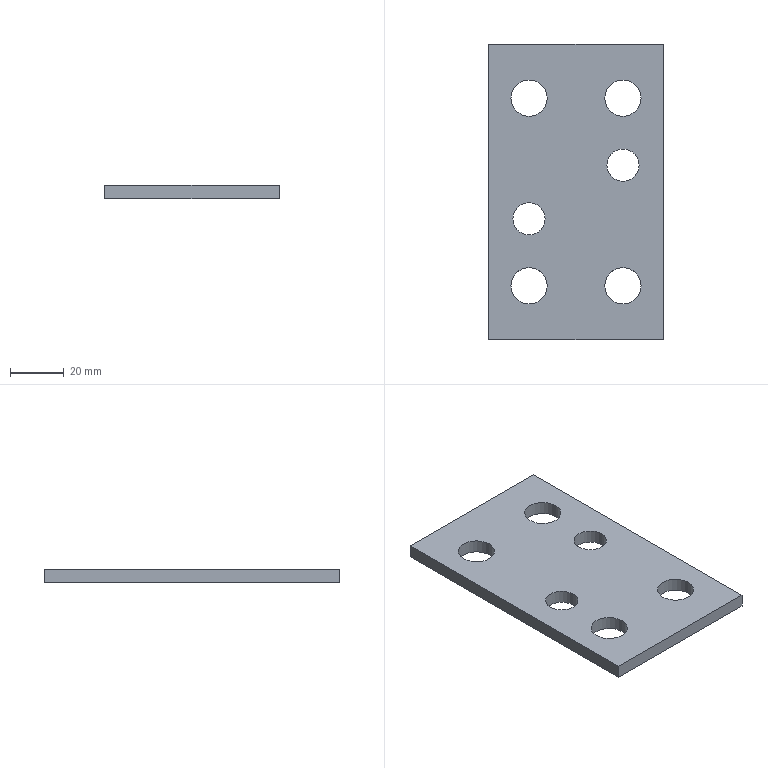Part | NX | features solid 2 | 1 solid | 12 faces | box 65 x 110 x 5 mm | volume 31756 mm3 | plane 6 | cylinder 6 | commonest cylinder face diameters 13.5 x4 12 x2
STEP:
#1=CARTESIAN_POINT('',(-997.,18.,70.));
#2=VERTEX_POINT('',#1);
#3=CARTESIAN_POINT('',(-1003.,18.,70.));
#4=DIRECTION('',(0.,0.,1.));
#5=DIRECTION('',(1.,0.,0.));
#6=AXIS2_PLACEMENT_3D('',#3,#4,#5);
#7=CIRCLE('',#6,6.);
#8=EDGE_CURVE('',#2,#2,#7,.F.);
#9=ORIENTED_EDGE('',*,*,#8,.F.);
#10=EDGE_LOOP('',(#9));
#11=FACE_BOUND('',#10,.T.);
#12=CARTESIAN_POINT('',(-1031.25,43.,70.));
#13=VERTEX_POINT('',#12);
#14=CARTESIAN_POINT('',(-1038.,43.,70.));
#15=DIRECTION('',(0.,0.,1.));
#16=DIRECTION('',(1.,0.,0.));
#17=AXIS2_PLACEMENT_3D('',#14,#15,#16);
#18=CIRCLE('',#17,6.75);
#19=EDGE_CURVE('',#13,#13,#18,.T.);
#20=ORIENTED_EDGE('',*,*,#19,.T.);
#21=EDGE_LOOP('',(#20));
#22=FACE_BOUND('',#21,.T.);
#23=CARTESIAN_POINT('',(-996.25,-27.,70.));
#24=VERTEX_POINT('',#23);
#25=CARTESIAN_POINT('',(-1003.,-27.,70.));
#26=DIRECTION('',(0.,0.,1.));
#27=DIRECTION('',(1.,0.,0.));
#28=AXIS2_PLACEMENT_3D('',#25,#26,#27);
#29=CIRCLE('',#28,6.75);
#30=EDGE_CURVE('',#24,#24,#29,.T.);
#31=ORIENTED_EDGE('',*,*,#30,.T.);
#32=EDGE_LOOP('',(#31));
#33=FACE_BOUND('',#32,.T.);
#34=CARTESIAN_POINT('',(-1053.,63.,70.));
#35=VERTEX_POINT('',#34);
#36=CARTESIAN_POINT('',(-988.,63.,70.));
#37=VERTEX_POINT('',#36);
#38=CARTESIAN_POINT('',(-1028.,63.,70.));
#39=DIRECTION('',(1.,0.,0.));
#40=VECTOR('',#39,1000.);
#41=LINE('',#38,#40);
#42=EDGE_CURVE('',#35,#37,#41,.T.);
#43=ORIENTED_EDGE('',*,*,#42,.T.);
#44=CARTESIAN_POINT('',(-988.,-47.,70.));
#45=VERTEX_POINT('',#44);
#46=CARTESIAN_POINT('',(-988.,8.,70.));
#47=DIRECTION('',(0.,-1.,0.));
#48=VECTOR('',#47,1000.);
#49=LINE('',#46,#48);
#50=EDGE_CURVE('',#37,#45,#49,.T.);
#51=ORIENTED_EDGE('',*,*,#50,.T.);
#52=CARTESIAN_POINT('',(-1053.,-47.,70.));
#53=VERTEX_POINT('',#52);
#54=CARTESIAN_POINT('',(-1028.,-47.,70.));
#55=DIRECTION('',(1.,0.,0.));
#56=VECTOR('',#55,1000.);
#57=LINE('',#54,#56);
#58=EDGE_CURVE('',#53,#45,#57,.T.);
#59=ORIENTED_EDGE('',*,*,#58,.F.);
#60=CARTESIAN_POINT('',(-1053.,8.,70.));
#61=DIRECTION('',(0.,-1.,0.));
#62=VECTOR('',#61,1000.);
#63=LINE('',#60,#62);
#64=EDGE_CURVE('',#35,#53,#63,.T.);
#65=ORIENTED_EDGE('',*,*,#64,.F.);
#66=EDGE_LOOP('',(#43,#51,#59,#65));
#67=FACE_BOUND('',#66,.T.);
#68=CARTESIAN_POINT('',(-1031.25,-27.,70.));
#69=VERTEX_POINT('',#68);
#70=CARTESIAN_POINT('',(-1038.,-27.,70.));
#71=DIRECTION('',(0.,0.,1.));
#72=DIRECTION('',(1.,0.,0.));
#73=AXIS2_PLACEMENT_3D('',#70,#71,#72);
#74=CIRCLE('',#73,6.75);
#75=EDGE_CURVE('',#69,#69,#74,.T.);
#76=ORIENTED_EDGE('',*,*,#75,.T.);
#77=EDGE_LOOP('',(#76));
#78=FACE_BOUND('',#77,.T.);
#79=CARTESIAN_POINT('',(-996.25,43.,70.));
#80=VERTEX_POINT('',#79);
#81=CARTESIAN_POINT('',(-1003.,43.,70.));
#82=DIRECTION('',(0.,0.,1.));
#83=DIRECTION('',(1.,0.,0.));
#84=AXIS2_PLACEMENT_3D('',#81,#82,#83);
#85=CIRCLE('',#84,6.75);
#86=EDGE_CURVE('',#80,#80,#85,.T.);
#87=ORIENTED_EDGE('',*,*,#86,.T.);
#88=EDGE_LOOP('',(#87));
#89=FACE_BOUND('',#88,.T.);
#90=CARTESIAN_POINT('',(-1032.,-2.,70.));
#91=VERTEX_POINT('',#90);
#92=CARTESIAN_POINT('',(-1038.,-2.,70.));
#93=DIRECTION('',(0.,0.,1.));
#94=DIRECTION('',(1.,0.,0.));
#95=AXIS2_PLACEMENT_3D('',#92,#93,#94);
#96=CIRCLE('',#95,6.);
#97=EDGE_CURVE('',#91,#91,#96,.F.);
#98=ORIENTED_EDGE('',*,*,#97,.F.);
#99=EDGE_LOOP('',(#98));
#100=FACE_BOUND('',#99,.T.);
#101=CARTESIAN_POINT('',(-1028.,8.,70.));
#102=DIRECTION('',(0.,0.,1.));
#103=DIRECTION('',(0.,-1.,0.));
#104=AXIS2_PLACEMENT_3D('',#101,#102,#103);
#105=PLANE('',#104);
#106=ADVANCED_FACE('',(#11,#22,#33,#67,#78,#89,#100),#105,.F.);
#107=CARTESIAN_POINT('',(-997.,18.,75.));
#108=VERTEX_POINT('',#107);
#109=CARTESIAN_POINT('',(-1003.,18.,75.));
#110=DIRECTION('',(0.,0.,1.));
#111=DIRECTION('',(1.,0.,0.));
#112=AXIS2_PLACEMENT_3D('',#109,#110,#111);
#113=CIRCLE('',#112,6.);
#114=EDGE_CURVE('',#108,#108,#113,.F.);
#115=ORIENTED_EDGE('',*,*,#114,.T.);
#116=EDGE_LOOP('',(#115));
#117=FACE_BOUND('',#116,.T.);
#118=CARTESIAN_POINT('',(-1031.25,43.,75.));
#119=VERTEX_POINT('',#118);
#120=CARTESIAN_POINT('',(-1038.,43.,75.));
#121=DIRECTION('',(0.,0.,1.));
#122=DIRECTION('',(1.,0.,0.));
#123=AXIS2_PLACEMENT_3D('',#120,#121,#122);
#124=CIRCLE('',#123,6.75);
#125=EDGE_CURVE('',#119,#119,#124,.T.);
#126=ORIENTED_EDGE('',*,*,#125,.F.);
#127=EDGE_LOOP('',(#126));
#128=FACE_BOUND('',#127,.T.);
#129=CARTESIAN_POINT('',(-996.25,-27.,75.));
#130=VERTEX_POINT('',#129);
#131=CARTESIAN_POINT('',(-1003.,-27.,75.));
#132=DIRECTION('',(0.,0.,1.));
#133=DIRECTION('',(1.,0.,0.));
#134=AXIS2_PLACEMENT_3D('',#131,#132,#133);
#135=CIRCLE('',#134,6.75);
#136=EDGE_CURVE('',#130,#130,#135,.T.);
#137=ORIENTED_EDGE('',*,*,#136,.F.);
#138=EDGE_LOOP('',(#137));
#139=FACE_BOUND('',#138,.T.);
#140=CARTESIAN_POINT('',(-1053.,63.,75.));
#141=VERTEX_POINT('',#140);
#142=CARTESIAN_POINT('',(-988.,63.,75.));
#143=VERTEX_POINT('',#142);
#144=CARTESIAN_POINT('',(-1028.,63.,75.));
#145=DIRECTION('',(1.,0.,0.));
#146=VECTOR('',#145,1000.);
#147=LINE('',#144,#146);
#148=EDGE_CURVE('',#141,#143,#147,.T.);
#149=ORIENTED_EDGE('',*,*,#148,.F.);
#150=CARTESIAN_POINT('',(-1053.,-47.,75.));
#151=VERTEX_POINT('',#150);
#152=CARTESIAN_POINT('',(-1053.,8.,75.));
#153=DIRECTION('',(0.,-1.,0.));
#154=VECTOR('',#153,1000.);
#155=LINE('',#152,#154);
#156=EDGE_CURVE('',#141,#151,#155,.T.);
#157=ORIENTED_EDGE('',*,*,#156,.T.);
#158=CARTESIAN_POINT('',(-988.,-47.,75.));
#159=VERTEX_POINT('',#158);
#160=CARTESIAN_POINT('',(-1028.,-47.,75.));
#161=DIRECTION('',(1.,0.,0.));
#162=VECTOR('',#161,1000.);
#163=LINE('',#160,#162);
#164=EDGE_CURVE('',#151,#159,#163,.T.);
#165=ORIENTED_EDGE('',*,*,#164,.T.);
#166=CARTESIAN_POINT('',(-988.,8.,75.));
#167=DIRECTION('',(0.,-1.,0.));
#168=VECTOR('',#167,1000.);
#169=LINE('',#166,#168);
#170=EDGE_CURVE('',#143,#159,#169,.T.);
#171=ORIENTED_EDGE('',*,*,#170,.F.);
#172=EDGE_LOOP('',(#149,#157,#165,#171));
#173=FACE_BOUND('',#172,.T.);
#174=CARTESIAN_POINT('',(-1031.25,-27.,75.));
#175=VERTEX_POINT('',#174);
#176=CARTESIAN_POINT('',(-1038.,-27.,75.));
#177=DIRECTION('',(0.,0.,1.));
#178=DIRECTION('',(1.,0.,0.));
#179=AXIS2_PLACEMENT_3D('',#176,#177,#178);
#180=CIRCLE('',#179,6.75);
#181=EDGE_CURVE('',#175,#175,#180,.T.);
#182=ORIENTED_EDGE('',*,*,#181,.F.);
#183=EDGE_LOOP('',(#182));
#184=FACE_BOUND('',#183,.T.);
#185=CARTESIAN_POINT('',(-996.25,43.,75.));
#186=VERTEX_POINT('',#185);
#187=CARTESIAN_POINT('',(-1003.,43.,75.));
#188=DIRECTION('',(0.,0.,1.));
#189=DIRECTION('',(1.,0.,0.));
#190=AXIS2_PLACEMENT_3D('',#187,#188,#189);
#191=CIRCLE('',#190,6.75);
#192=EDGE_CURVE('',#186,#186,#191,.T.);
#193=ORIENTED_EDGE('',*,*,#192,.F.);
#194=EDGE_LOOP('',(#193));
#195=FACE_BOUND('',#194,.T.);
#196=CARTESIAN_POINT('',(-1032.,-2.,75.));
#197=VERTEX_POINT('',#196);
#198=CARTESIAN_POINT('',(-1038.,-2.,75.));
#199=DIRECTION('',(0.,0.,1.));
#200=DIRECTION('',(1.,0.,0.));
#201=AXIS2_PLACEMENT_3D('',#198,#199,#200);
#202=CIRCLE('',#201,6.);
#203=EDGE_CURVE('',#197,#197,#202,.F.);
#204=ORIENTED_EDGE('',*,*,#203,.T.);
#205=EDGE_LOOP('',(#204));
#206=FACE_BOUND('',#205,.T.);
#207=CARTESIAN_POINT('',(-1028.,8.,75.));
#208=DIRECTION('',(0.,0.,1.));
#209=DIRECTION('',(0.,-1.,0.));
#210=AXIS2_PLACEMENT_3D('',#207,#208,#209);
#211=PLANE('',#210);
#212=ADVANCED_FACE('',(#117,#128,#139,#173,#184,#195,#206),#211,.T.);
#213=ORIENTED_EDGE('',*,*,#148,.T.);
#214=CARTESIAN_POINT('',(-988.,63.,70.));
#215=DIRECTION('',(0.,0.,1.));
#216=VECTOR('',#215,1000.);
#217=LINE('',#214,#216);
#218=EDGE_CURVE('',#37,#143,#217,.T.);
#219=ORIENTED_EDGE('',*,*,#218,.F.);
#220=ORIENTED_EDGE('',*,*,#42,.F.);
#221=CARTESIAN_POINT('',(-1053.,63.,70.));
#222=DIRECTION('',(0.,0.,1.));
#223=VECTOR('',#222,1000.);
#224=LINE('',#221,#223);
#225=EDGE_CURVE('',#35,#141,#224,.T.);
#226=ORIENTED_EDGE('',*,*,#225,.T.);
#227=EDGE_LOOP('',(#213,#219,#220,#226));
#228=FACE_BOUND('',#227,.T.);
#229=CARTESIAN_POINT('',(-1028.,63.,70.));
#230=DIRECTION('',(0.,-1.,0.));
#231=DIRECTION('',(0.,0.,-1.));
#232=AXIS2_PLACEMENT_3D('',#229,#230,#231);
#233=PLANE('',#232);
#234=ADVANCED_FACE('',(#228),#233,.F.);
#235=ORIENTED_EDGE('',*,*,#156,.F.);
#236=ORIENTED_EDGE('',*,*,#225,.F.);
#237=ORIENTED_EDGE('',*,*,#64,.T.);
#238=CARTESIAN_POINT('',(-1053.,-47.,70.));
#239=DIRECTION('',(0.,0.,1.));
#240=VECTOR('',#239,1000.);
#241=LINE('',#238,#240);
#242=EDGE_CURVE('',#53,#151,#241,.T.);
#243=ORIENTED_EDGE('',*,*,#242,.T.);
#244=EDGE_LOOP('',(#235,#236,#237,#243));
#245=FACE_BOUND('',#244,.T.);
#246=CARTESIAN_POINT('',(-1053.,8.,70.));
#247=DIRECTION('',(-1.,0.,0.));
#248=DIRECTION('',(0.,0.,1.));
#249=AXIS2_PLACEMENT_3D('',#246,#247,#248);
#250=PLANE('',#249);
#251=ADVANCED_FACE('',(#245),#250,.T.);
#252=ORIENTED_EDGE('',*,*,#164,.F.);
#253=ORIENTED_EDGE('',*,*,#242,.F.);
#254=ORIENTED_EDGE('',*,*,#58,.T.);
#255=CARTESIAN_POINT('',(-988.,-47.,70.));
#256=DIRECTION('',(0.,0.,1.));
#257=VECTOR('',#256,1000.);
#258=LINE('',#255,#257);
#259=EDGE_CURVE('',#45,#159,#258,.T.);
#260=ORIENTED_EDGE('',*,*,#259,.T.);
#261=EDGE_LOOP('',(#252,#253,#254,#260));
#262=FACE_BOUND('',#261,.T.);
#263=CARTESIAN_POINT('',(-1028.,-47.,70.));
#264=DIRECTION('',(0.,-1.,0.));
#265=DIRECTION('',(0.,0.,-1.));
#266=AXIS2_PLACEMENT_3D('',#263,#264,#265);
#267=PLANE('',#266);
#268=ADVANCED_FACE('',(#262),#267,.T.);
#269=ORIENTED_EDGE('',*,*,#75,.F.);
#270=EDGE_LOOP('',(#269));
#271=FACE_BOUND('',#270,.T.);
#272=ORIENTED_EDGE('',*,*,#181,.T.);
#273=EDGE_LOOP('',(#272));
#274=FACE_BOUND('',#273,.T.);
#275=CARTESIAN_POINT('',(-1038.,-27.,70.));
#276=DIRECTION('',(0.,0.,1.));
#277=DIRECTION('',(1.,0.,0.));
#278=AXIS2_PLACEMENT_3D('',#275,#276,#277);
#279=CYLINDRICAL_SURFACE('',#278,6.75);
#280=ADVANCED_FACE('',(#271,#274),#279,.F.);
#281=ORIENTED_EDGE('',*,*,#170,.T.);
#282=ORIENTED_EDGE('',*,*,#259,.F.);
#283=ORIENTED_EDGE('',*,*,#50,.F.);
#284=ORIENTED_EDGE('',*,*,#218,.T.);
#285=EDGE_LOOP('',(#281,#282,#283,#284));
#286=FACE_BOUND('',#285,.T.);
#287=CARTESIAN_POINT('',(-988.,8.,70.));
#288=DIRECTION('',(-1.,0.,0.));
#289=DIRECTION('',(0.,0.,1.));
#290=AXIS2_PLACEMENT_3D('',#287,#288,#289);
#291=PLANE('',#290);
#292=ADVANCED_FACE('',(#286),#291,.F.);
#293=ORIENTED_EDGE('',*,*,#30,.F.);
#294=EDGE_LOOP('',(#293));
#295=FACE_BOUND('',#294,.T.);
#296=ORIENTED_EDGE('',*,*,#136,.T.);
#297=EDGE_LOOP('',(#296));
#298=FACE_BOUND('',#297,.T.);
#299=CARTESIAN_POINT('',(-1003.,-27.,70.));
#300=DIRECTION('',(0.,0.,1.));
#301=DIRECTION('',(1.,0.,0.));
#302=AXIS2_PLACEMENT_3D('',#299,#300,#301);
#303=CYLINDRICAL_SURFACE('',#302,6.75);
#304=ADVANCED_FACE('',(#295,#298),#303,.F.);
#305=ORIENTED_EDGE('',*,*,#19,.F.);
#306=EDGE_LOOP('',(#305));
#307=FACE_BOUND('',#306,.T.);
#308=ORIENTED_EDGE('',*,*,#125,.T.);
#309=EDGE_LOOP('',(#308));
#310=FACE_BOUND('',#309,.T.);
#311=CARTESIAN_POINT('',(-1038.,43.,70.));
#312=DIRECTION('',(0.,0.,1.));
#313=DIRECTION('',(1.,0.,0.));
#314=AXIS2_PLACEMENT_3D('',#311,#312,#313);
#315=CYLINDRICAL_SURFACE('',#314,6.75);
#316=ADVANCED_FACE('',(#307,#310),#315,.F.);
#317=ORIENTED_EDGE('',*,*,#86,.F.);
#318=EDGE_LOOP('',(#317));
#319=FACE_BOUND('',#318,.T.);
#320=ORIENTED_EDGE('',*,*,#192,.T.);
#321=EDGE_LOOP('',(#320));
#322=FACE_BOUND('',#321,.T.);
#323=CARTESIAN_POINT('',(-1003.,43.,70.));
#324=DIRECTION('',(0.,0.,1.));
#325=DIRECTION('',(1.,0.,0.));
#326=AXIS2_PLACEMENT_3D('',#323,#324,#325);
#327=CYLINDRICAL_SURFACE('',#326,6.75);
#328=ADVANCED_FACE('',(#319,#322),#327,.F.);
#329=ORIENTED_EDGE('',*,*,#114,.F.);
#330=EDGE_LOOP('',(#329));
#331=FACE_BOUND('',#330,.T.);
#332=ORIENTED_EDGE('',*,*,#8,.T.);
#333=EDGE_LOOP('',(#332));
#334=FACE_BOUND('',#333,.T.);
#335=CARTESIAN_POINT('',(-1003.,18.,550.));
#336=DIRECTION('',(0.,0.,-1.));
#337=DIRECTION('',(-1.,0.,0.));
#338=AXIS2_PLACEMENT_3D('',#335,#336,#337);
#339=CYLINDRICAL_SURFACE('',#338,6.);
#340=ADVANCED_FACE('',(#331,#334),#339,.F.);
#341=ORIENTED_EDGE('',*,*,#203,.F.);
#342=EDGE_LOOP('',(#341));
#343=FACE_BOUND('',#342,.T.);
#344=ORIENTED_EDGE('',*,*,#97,.T.);
#345=EDGE_LOOP('',(#344));
#346=FACE_BOUND('',#345,.T.);
#347=CARTESIAN_POINT('',(-1038.,-2.,550.));
#348=DIRECTION('',(0.,0.,-1.));
#349=DIRECTION('',(-1.,0.,0.));
#350=AXIS2_PLACEMENT_3D('',#347,#348,#349);
#351=CYLINDRICAL_SURFACE('',#350,6.);
#352=ADVANCED_FACE('',(#343,#346),#351,.F.);
#353=CLOSED_SHELL('',(#106,#212,#234,#251,#268,#280,#292,#304,#316,#328,#340,#352));
#354=MANIFOLD_SOLID_BREP('',#353);
#355=(LENGTH_UNIT()NAMED_UNIT(*)SI_UNIT(.MILLI.,.METRE.));
#356=UNCERTAINTY_MEASURE_WITH_UNIT(LENGTH_MEASURE(0.00001),#355,'','');
#357=(NAMED_UNIT(*)PLANE_ANGLE_UNIT()SI_UNIT($,.RADIAN.));
#358=(NAMED_UNIT(*)SI_UNIT($,.STERADIAN.)SOLID_ANGLE_UNIT());
#359=(GEOMETRIC_REPRESENTATION_CONTEXT(3)GLOBAL_UNCERTAINTY_ASSIGNED_CONTEXT((#356))GLOBAL_UNIT_ASSIGNED_CONTEXT((#355,#357,#358))REPRESENTATION_CONTEXT('',''));
#360=ADVANCED_BREP_SHAPE_REPRESENTATION('',(#354),#359);